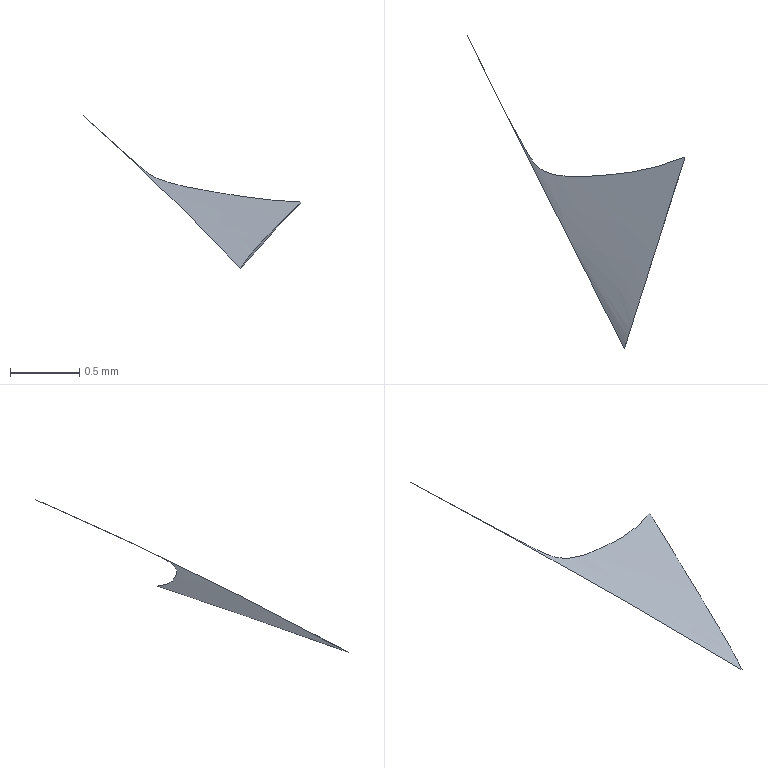Part | Creo | 1 solid | 3 faces | box 1.577 x 2.258 x 1.103 mm | volume 0.003877 mm3 | cone 1 | plane 1 | spline 1